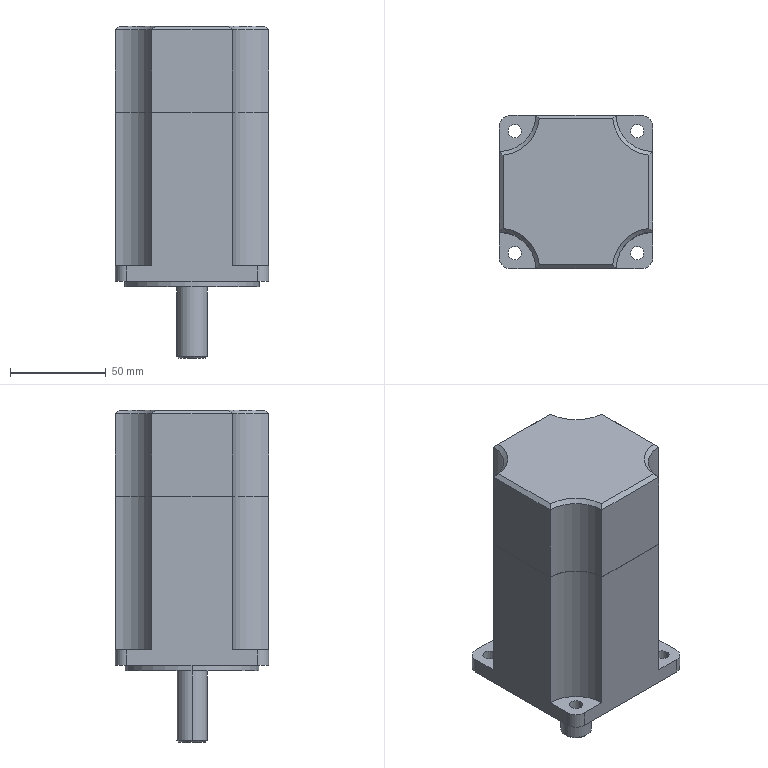Part | STEP file | 1FL40-44-0AF21-0AA0 | 2 solids | 52 faces | box 80 x 80 x 173 mm | volume 725829 mm3 | cylinder 24 | plane 22 | cone 6 | commonest cylinder face diameters 7 x8 38 x8 12 x4 16 x2 70 x2